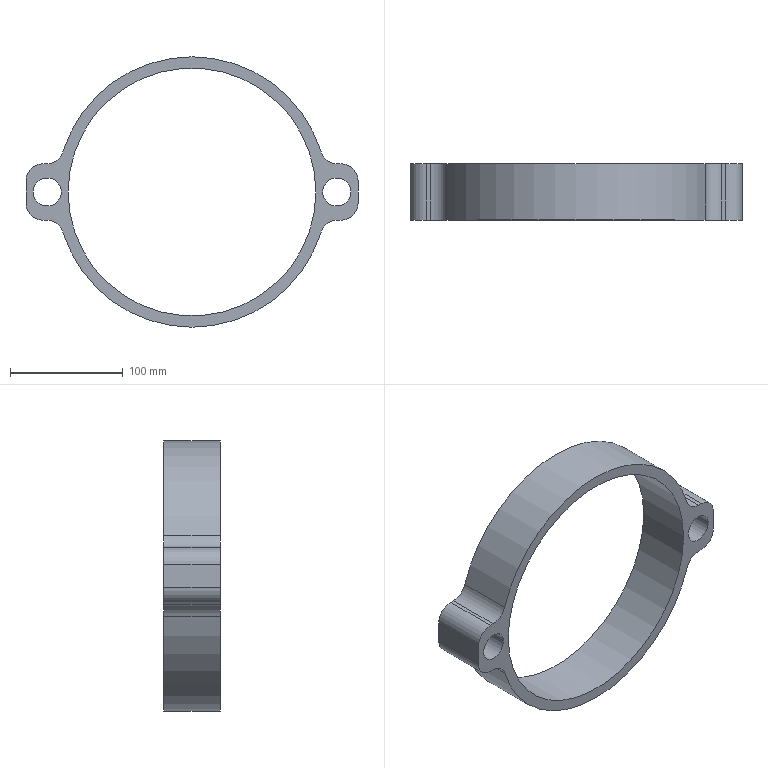Part | NX | features BREP 1 | 1 solid | 24 faces | box 294.734 x 50 x 240 mm | volume 448691 mm3 | cylinder 16 | plane 8 | commonest cylinder face diameters 30 x8 25 x4 220 x2 240 x2
STEP:
#1=CARTESIAN_POINT('',(-128.938,0.,-25.));
#2=VERTEX_POINT('',#1);
#3=CARTESIAN_POINT('',(-132.367,0.,-25.));
#4=VERTEX_POINT('',#3);
#5=CARTESIAN_POINT('',(-128.938,0.,-25.));
#6=DIRECTION('',(-1.,0.,0.));
#7=VECTOR('',#6,1000.);
#8=LINE('',#5,#7);
#9=EDGE_CURVE('',#2,#4,#8,.T.);
#10=ORIENTED_EDGE('',*,*,#9,.F.);
#11=CARTESIAN_POINT('',(-114.612,0.,-35.556));
#12=VERTEX_POINT('',#11);
#13=CARTESIAN_POINT('',(-128.938,0.,-40.));
#14=DIRECTION('',(0.,1.,0.));
#15=DIRECTION('',(0.,0.,1.));
#16=AXIS2_PLACEMENT_3D('',#13,#14,#15);
#17=CIRCLE('',#16,15.);
#18=EDGE_CURVE('',#2,#12,#17,.T.);
#19=ORIENTED_EDGE('',*,*,#18,.T.);
#20=CARTESIAN_POINT('',(114.612,0.,-35.556));
#21=VERTEX_POINT('',#20);
#22=CARTESIAN_POINT('',(0.,0.,0.));
#23=DIRECTION('',(0.,1.,0.));
#24=DIRECTION('',(0.9551,0.,-0.2963));
#25=AXIS2_PLACEMENT_3D('',#22,#23,#24);
#26=CIRCLE('',#25,120.);
#27=EDGE_CURVE('',#21,#12,#26,.T.);
#28=ORIENTED_EDGE('',*,*,#27,.F.);
#29=CARTESIAN_POINT('',(128.938,0.,-25.));
#30=VERTEX_POINT('',#29);
#31=CARTESIAN_POINT('',(128.938,0.,-40.));
#32=DIRECTION('',(0.,1.,0.));
#33=DIRECTION('',(-0.9551,0.,0.2963));
#34=AXIS2_PLACEMENT_3D('',#31,#32,#33);
#35=CIRCLE('',#34,15.);
#36=EDGE_CURVE('',#21,#30,#35,.T.);
#37=ORIENTED_EDGE('',*,*,#36,.T.);
#38=CARTESIAN_POINT('',(132.367,0.,-25.));
#39=VERTEX_POINT('',#38);
#40=CARTESIAN_POINT('',(132.367,0.,-25.));
#41=DIRECTION('',(-1.,0.,0.));
#42=VECTOR('',#41,1000.);
#43=LINE('',#40,#42);
#44=EDGE_CURVE('',#39,#30,#43,.T.);
#45=ORIENTED_EDGE('',*,*,#44,.F.);
#46=CARTESIAN_POINT('',(147.367,0.,-10.));
#47=VERTEX_POINT('',#46);
#48=CARTESIAN_POINT('',(132.367,0.,-10.));
#49=DIRECTION('',(0.,-1.,0.));
#50=DIRECTION('',(0.,0.,-1.));
#51=AXIS2_PLACEMENT_3D('',#48,#49,#50);
#52=CIRCLE('',#51,15.);
#53=EDGE_CURVE('',#39,#47,#52,.T.);
#54=ORIENTED_EDGE('',*,*,#53,.T.);
#55=CARTESIAN_POINT('',(147.367,0.,10.));
#56=VERTEX_POINT('',#55);
#57=CARTESIAN_POINT('',(147.367,0.,10.));
#58=DIRECTION('',(0.,0.,-1.));
#59=VECTOR('',#58,1000.);
#60=LINE('',#57,#59);
#61=EDGE_CURVE('',#56,#47,#60,.T.);
#62=ORIENTED_EDGE('',*,*,#61,.F.);
#63=CARTESIAN_POINT('',(132.367,0.,25.));
#64=VERTEX_POINT('',#63);
#65=CARTESIAN_POINT('',(132.367,0.,10.));
#66=DIRECTION('',(0.,-1.,0.));
#67=DIRECTION('',(1.,0.,0.));
#68=AXIS2_PLACEMENT_3D('',#65,#66,#67);
#69=CIRCLE('',#68,15.);
#70=EDGE_CURVE('',#56,#64,#69,.T.);
#71=ORIENTED_EDGE('',*,*,#70,.T.);
#72=CARTESIAN_POINT('',(128.938,0.,25.));
#73=VERTEX_POINT('',#72);
#74=CARTESIAN_POINT('',(128.938,0.,25.));
#75=DIRECTION('',(1.,0.,0.));
#76=VECTOR('',#75,1000.);
#77=LINE('',#74,#76);
#78=EDGE_CURVE('',#73,#64,#77,.T.);
#79=ORIENTED_EDGE('',*,*,#78,.F.);
#80=CARTESIAN_POINT('',(114.612,0.,35.556));
#81=VERTEX_POINT('',#80);
#82=CARTESIAN_POINT('',(128.938,0.,40.));
#83=DIRECTION('',(0.,1.,0.));
#84=DIRECTION('',(0.,0.,-1.));
#85=AXIS2_PLACEMENT_3D('',#82,#83,#84);
#86=CIRCLE('',#85,15.);
#87=EDGE_CURVE('',#73,#81,#86,.T.);
#88=ORIENTED_EDGE('',*,*,#87,.T.);
#89=CARTESIAN_POINT('',(-114.612,0.,35.556));
#90=VERTEX_POINT('',#89);
#91=CARTESIAN_POINT('',(0.,0.,0.));
#92=DIRECTION('',(0.,1.,0.));
#93=DIRECTION('',(-0.9551,0.,0.2963));
#94=AXIS2_PLACEMENT_3D('',#91,#92,#93);
#95=CIRCLE('',#94,120.);
#96=EDGE_CURVE('',#90,#81,#95,.T.);
#97=ORIENTED_EDGE('',*,*,#96,.F.);
#98=CARTESIAN_POINT('',(-128.938,0.,25.));
#99=VERTEX_POINT('',#98);
#100=CARTESIAN_POINT('',(-128.938,0.,40.));
#101=DIRECTION('',(0.,1.,0.));
#102=DIRECTION('',(0.9551,0.,-0.2963));
#103=AXIS2_PLACEMENT_3D('',#100,#101,#102);
#104=CIRCLE('',#103,15.);
#105=EDGE_CURVE('',#90,#99,#104,.T.);
#106=ORIENTED_EDGE('',*,*,#105,.T.);
#107=CARTESIAN_POINT('',(-132.367,0.,25.));
#108=VERTEX_POINT('',#107);
#109=CARTESIAN_POINT('',(-132.367,0.,25.));
#110=DIRECTION('',(1.,0.,0.));
#111=VECTOR('',#110,1000.);
#112=LINE('',#109,#111);
#113=EDGE_CURVE('',#108,#99,#112,.T.);
#114=ORIENTED_EDGE('',*,*,#113,.F.);
#115=CARTESIAN_POINT('',(-147.367,0.,10.));
#116=VERTEX_POINT('',#115);
#117=CARTESIAN_POINT('',(-132.367,0.,10.));
#118=DIRECTION('',(0.,-1.,0.));
#119=DIRECTION('',(0.,0.,1.));
#120=AXIS2_PLACEMENT_3D('',#117,#118,#119);
#121=CIRCLE('',#120,15.);
#122=EDGE_CURVE('',#108,#116,#121,.T.);
#123=ORIENTED_EDGE('',*,*,#122,.T.);
#124=CARTESIAN_POINT('',(-147.367,0.,-10.));
#125=VERTEX_POINT('',#124);
#126=CARTESIAN_POINT('',(-147.367,0.,-10.));
#127=DIRECTION('',(0.,0.,1.));
#128=VECTOR('',#127,1000.);
#129=LINE('',#126,#128);
#130=EDGE_CURVE('',#125,#116,#129,.T.);
#131=ORIENTED_EDGE('',*,*,#130,.F.);
#132=CARTESIAN_POINT('',(-132.367,0.,-10.));
#133=DIRECTION('',(0.,-1.,0.));
#134=DIRECTION('',(-1.,0.,0.));
#135=AXIS2_PLACEMENT_3D('',#132,#133,#134);
#136=CIRCLE('',#135,15.);
#137=EDGE_CURVE('',#125,#4,#136,.T.);
#138=ORIENTED_EDGE('',*,*,#137,.T.);
#139=EDGE_LOOP('',(#10,#19,#28,#37,#45,#54,#62,#71,#79,#88,#97,#106,#114,#123,#131,#138));
#140=FACE_BOUND('',#139,.T.);
#141=CARTESIAN_POINT('',(-110.,0.,0.));
#142=VERTEX_POINT('',#141);
#143=CARTESIAN_POINT('',(110.,0.,0.));
#144=VERTEX_POINT('',#143);
#145=CARTESIAN_POINT('',(0.,0.,0.));
#146=DIRECTION('',(0.,-1.,0.));
#147=DIRECTION('',(-1.,0.,0.));
#148=AXIS2_PLACEMENT_3D('',#145,#146,#147);
#149=CIRCLE('',#148,110.);
#150=EDGE_CURVE('',#142,#144,#149,.T.);
#151=ORIENTED_EDGE('',*,*,#150,.F.);
#152=CARTESIAN_POINT('',(0.,0.,0.));
#153=DIRECTION('',(0.,-1.,0.));
#154=DIRECTION('',(1.,0.,0.));
#155=AXIS2_PLACEMENT_3D('',#152,#153,#154);
#156=CIRCLE('',#155,110.);
#157=EDGE_CURVE('',#144,#142,#156,.T.);
#158=ORIENTED_EDGE('',*,*,#157,.F.);
#159=EDGE_LOOP('',(#151,#158));
#160=FACE_BOUND('',#159,.T.);
#161=CARTESIAN_POINT('',(-141.,0.,0.));
#162=VERTEX_POINT('',#161);
#163=CARTESIAN_POINT('',(-116.,0.,0.));
#164=VERTEX_POINT('',#163);
#165=CARTESIAN_POINT('',(-128.5,0.,0.));
#166=DIRECTION('',(0.,1.,0.));
#167=DIRECTION('',(-1.,0.,0.));
#168=AXIS2_PLACEMENT_3D('',#165,#166,#167);
#169=CIRCLE('',#168,12.5);
#170=EDGE_CURVE('',#162,#164,#169,.T.);
#171=ORIENTED_EDGE('',*,*,#170,.T.);
#172=CARTESIAN_POINT('',(-128.5,0.,0.));
#173=DIRECTION('',(0.,1.,0.));
#174=DIRECTION('',(1.,0.,0.));
#175=AXIS2_PLACEMENT_3D('',#172,#173,#174);
#176=CIRCLE('',#175,12.5);
#177=EDGE_CURVE('',#164,#162,#176,.T.);
#178=ORIENTED_EDGE('',*,*,#177,.T.);
#179=EDGE_LOOP('',(#171,#178));
#180=FACE_BOUND('',#179,.T.);
#181=CARTESIAN_POINT('',(116.,0.,0.));
#182=VERTEX_POINT('',#181);
#183=CARTESIAN_POINT('',(141.,0.,0.));
#184=VERTEX_POINT('',#183);
#185=CARTESIAN_POINT('',(128.5,0.,0.));
#186=DIRECTION('',(0.,1.,0.));
#187=DIRECTION('',(-1.,0.,0.));
#188=AXIS2_PLACEMENT_3D('',#185,#186,#187);
#189=CIRCLE('',#188,12.5);
#190=EDGE_CURVE('',#182,#184,#189,.T.);
#191=ORIENTED_EDGE('',*,*,#190,.T.);
#192=CARTESIAN_POINT('',(128.5,0.,0.));
#193=DIRECTION('',(0.,1.,0.));
#194=DIRECTION('',(1.,0.,0.));
#195=AXIS2_PLACEMENT_3D('',#192,#193,#194);
#196=CIRCLE('',#195,12.5);
#197=EDGE_CURVE('',#184,#182,#196,.T.);
#198=ORIENTED_EDGE('',*,*,#197,.T.);
#199=EDGE_LOOP('',(#191,#198));
#200=FACE_BOUND('',#199,.T.);
#201=CARTESIAN_POINT('',(0.,0.,0.));
#202=DIRECTION('',(0.,1.,0.));
#203=DIRECTION('',(1.,0.,0.));
#204=AXIS2_PLACEMENT_3D('',#201,#202,#203);
#205=PLANE('',#204);
#206=ADVANCED_FACE('',(#140,#160,#180,#200),#205,.F.);
#207=CARTESIAN_POINT('',(-110.,50.,0.));
#208=VERTEX_POINT('',#207);
#209=CARTESIAN_POINT('',(-110.,0.,0.));
#210=DIRECTION('',(0.,1.,0.));
#211=VECTOR('',#210,1000.);
#212=LINE('',#209,#211);
#213=EDGE_CURVE('',#142,#208,#212,.T.);
#214=ORIENTED_EDGE('',*,*,#213,.T.);
#215=CARTESIAN_POINT('',(110.,50.,0.));
#216=VERTEX_POINT('',#215);
#217=CARTESIAN_POINT('',(0.,50.,0.));
#218=DIRECTION('',(0.,-1.,0.));
#219=DIRECTION('',(1.,0.,0.));
#220=AXIS2_PLACEMENT_3D('',#217,#218,#219);
#221=CIRCLE('',#220,110.);
#222=EDGE_CURVE('',#216,#208,#221,.T.);
#223=ORIENTED_EDGE('',*,*,#222,.F.);
#224=CARTESIAN_POINT('',(110.,0.,0.));
#225=DIRECTION('',(0.,1.,0.));
#226=VECTOR('',#225,1000.);
#227=LINE('',#224,#226);
#228=EDGE_CURVE('',#144,#216,#227,.T.);
#229=ORIENTED_EDGE('',*,*,#228,.F.);
#230=ORIENTED_EDGE('',*,*,#157,.T.);
#231=EDGE_LOOP('',(#214,#223,#229,#230));
#232=FACE_BOUND('',#231,.T.);
#233=CARTESIAN_POINT('',(0.,0.,0.));
#234=DIRECTION('',(0.,1.,0.));
#235=DIRECTION('',(1.,0.,0.));
#236=AXIS2_PLACEMENT_3D('',#233,#234,#235);
#237=CYLINDRICAL_SURFACE('',#236,110.);
#238=ADVANCED_FACE('',(#232),#237,.F.);
#239=ORIENTED_EDGE('',*,*,#228,.T.);
#240=CARTESIAN_POINT('',(0.,50.,0.));
#241=DIRECTION('',(0.,-1.,0.));
#242=DIRECTION('',(-1.,0.,0.));
#243=AXIS2_PLACEMENT_3D('',#240,#241,#242);
#244=CIRCLE('',#243,110.);
#245=EDGE_CURVE('',#208,#216,#244,.T.);
#246=ORIENTED_EDGE('',*,*,#245,.F.);
#247=ORIENTED_EDGE('',*,*,#213,.F.);
#248=ORIENTED_EDGE('',*,*,#150,.T.);
#249=EDGE_LOOP('',(#239,#246,#247,#248));
#250=FACE_BOUND('',#249,.T.);
#251=CARTESIAN_POINT('',(0.,0.,0.));
#252=DIRECTION('',(0.,1.,0.));
#253=DIRECTION('',(1.,0.,0.));
#254=AXIS2_PLACEMENT_3D('',#251,#252,#253);
#255=CYLINDRICAL_SURFACE('',#254,110.);
#256=ADVANCED_FACE('',(#250),#255,.F.);
#257=CARTESIAN_POINT('',(-147.367,50.,-10.));
#258=VERTEX_POINT('',#257);
#259=CARTESIAN_POINT('',(-147.367,50.,10.));
#260=VERTEX_POINT('',#259);
#261=CARTESIAN_POINT('',(-147.367,50.,-10.));
#262=DIRECTION('',(0.,0.,1.));
#263=VECTOR('',#262,1000.);
#264=LINE('',#261,#263);
#265=EDGE_CURVE('',#258,#260,#264,.T.);
#266=ORIENTED_EDGE('',*,*,#265,.T.);
#267=CARTESIAN_POINT('',(-132.367,50.,25.));
#268=VERTEX_POINT('',#267);
#269=CARTESIAN_POINT('',(-132.367,50.,10.));
#270=DIRECTION('',(0.,1.,0.));
#271=DIRECTION('',(-1.,0.,0.));
#272=AXIS2_PLACEMENT_3D('',#269,#270,#271);
#273=CIRCLE('',#272,15.);
#274=EDGE_CURVE('',#260,#268,#273,.T.);
#275=ORIENTED_EDGE('',*,*,#274,.T.);
#276=CARTESIAN_POINT('',(-128.938,50.,25.));
#277=VERTEX_POINT('',#276);
#278=CARTESIAN_POINT('',(-132.367,50.,25.));
#279=DIRECTION('',(1.,0.,0.));
#280=VECTOR('',#279,1000.);
#281=LINE('',#278,#280);
#282=EDGE_CURVE('',#268,#277,#281,.T.);
#283=ORIENTED_EDGE('',*,*,#282,.T.);
#284=CARTESIAN_POINT('',(-114.612,50.,35.556));
#285=VERTEX_POINT('',#284);
#286=CARTESIAN_POINT('',(-128.938,50.,40.));
#287=DIRECTION('',(0.,-1.,0.));
#288=DIRECTION('',(0.,0.,-1.));
#289=AXIS2_PLACEMENT_3D('',#286,#287,#288);
#290=CIRCLE('',#289,15.);
#291=EDGE_CURVE('',#277,#285,#290,.T.);
#292=ORIENTED_EDGE('',*,*,#291,.T.);
#293=CARTESIAN_POINT('',(114.612,50.,35.556));
#294=VERTEX_POINT('',#293);
#295=CARTESIAN_POINT('',(0.,50.,0.));
#296=DIRECTION('',(0.,1.,0.));
#297=DIRECTION('',(-0.9551,0.,0.2963));
#298=AXIS2_PLACEMENT_3D('',#295,#296,#297);
#299=CIRCLE('',#298,120.);
#300=EDGE_CURVE('',#285,#294,#299,.T.);
#301=ORIENTED_EDGE('',*,*,#300,.T.);
#302=CARTESIAN_POINT('',(128.938,50.,25.));
#303=VERTEX_POINT('',#302);
#304=CARTESIAN_POINT('',(128.938,50.,40.));
#305=DIRECTION('',(0.,-1.,0.));
#306=DIRECTION('',(-0.9551,0.,-0.2963));
#307=AXIS2_PLACEMENT_3D('',#304,#305,#306);
#308=CIRCLE('',#307,15.);
#309=EDGE_CURVE('',#294,#303,#308,.T.);
#310=ORIENTED_EDGE('',*,*,#309,.T.);
#311=CARTESIAN_POINT('',(132.367,50.,25.));
#312=VERTEX_POINT('',#311);
#313=CARTESIAN_POINT('',(128.938,50.,25.));
#314=DIRECTION('',(1.,0.,0.));
#315=VECTOR('',#314,1000.);
#316=LINE('',#313,#315);
#317=EDGE_CURVE('',#303,#312,#316,.T.);
#318=ORIENTED_EDGE('',*,*,#317,.T.);
#319=CARTESIAN_POINT('',(147.367,50.,10.));
#320=VERTEX_POINT('',#319);
#321=CARTESIAN_POINT('',(132.367,50.,10.));
#322=DIRECTION('',(0.,1.,0.));
#323=DIRECTION('',(0.,0.,1.));
#324=AXIS2_PLACEMENT_3D('',#321,#322,#323);
#325=CIRCLE('',#324,15.);
#326=EDGE_CURVE('',#312,#320,#325,.T.);
#327=ORIENTED_EDGE('',*,*,#326,.T.);
#328=CARTESIAN_POINT('',(147.367,50.,-10.));
#329=VERTEX_POINT('',#328);
#330=CARTESIAN_POINT('',(147.367,50.,10.));
#331=DIRECTION('',(0.,0.,-1.));
#332=VECTOR('',#331,1000.);
#333=LINE('',#330,#332);
#334=EDGE_CURVE('',#320,#329,#333,.T.);
#335=ORIENTED_EDGE('',*,*,#334,.T.);
#336=CARTESIAN_POINT('',(132.367,50.,-25.));
#337=VERTEX_POINT('',#336);
#338=CARTESIAN_POINT('',(132.367,50.,-10.));
#339=DIRECTION('',(0.,1.,0.));
#340=DIRECTION('',(1.,0.,0.));
#341=AXIS2_PLACEMENT_3D('',#338,#339,#340);
#342=CIRCLE('',#341,15.);
#343=EDGE_CURVE('',#329,#337,#342,.T.);
#344=ORIENTED_EDGE('',*,*,#343,.T.);
#345=CARTESIAN_POINT('',(128.938,50.,-25.));
#346=VERTEX_POINT('',#345);
#347=CARTESIAN_POINT('',(132.367,50.,-25.));
#348=DIRECTION('',(-1.,0.,0.));
#349=VECTOR('',#348,1000.);
#350=LINE('',#347,#349);
#351=EDGE_CURVE('',#337,#346,#350,.T.);
#352=ORIENTED_EDGE('',*,*,#351,.T.);
#353=CARTESIAN_POINT('',(114.612,50.,-35.556));
#354=VERTEX_POINT('',#353);
#355=CARTESIAN_POINT('',(128.938,50.,-40.));
#356=DIRECTION('',(0.,-1.,0.));
#357=DIRECTION('',(0.,0.,1.));
#358=AXIS2_PLACEMENT_3D('',#355,#356,#357);
#359=CIRCLE('',#358,15.);
#360=EDGE_CURVE('',#346,#354,#359,.T.);
#361=ORIENTED_EDGE('',*,*,#360,.T.);
#362=CARTESIAN_POINT('',(-114.612,50.,-35.556));
#363=VERTEX_POINT('',#362);
#364=CARTESIAN_POINT('',(0.,50.,0.));
#365=DIRECTION('',(0.,1.,0.));
#366=DIRECTION('',(0.9551,0.,-0.2963));
#367=AXIS2_PLACEMENT_3D('',#364,#365,#366);
#368=CIRCLE('',#367,120.);
#369=EDGE_CURVE('',#354,#363,#368,.T.);
#370=ORIENTED_EDGE('',*,*,#369,.T.);
#371=CARTESIAN_POINT('',(-128.938,50.,-25.));
#372=VERTEX_POINT('',#371);
#373=CARTESIAN_POINT('',(-128.938,50.,-40.));
#374=DIRECTION('',(0.,-1.,0.));
#375=DIRECTION('',(0.9551,0.,0.2963));
#376=AXIS2_PLACEMENT_3D('',#373,#374,#375);
#377=CIRCLE('',#376,15.);
#378=EDGE_CURVE('',#363,#372,#377,.T.);
#379=ORIENTED_EDGE('',*,*,#378,.T.);
#380=CARTESIAN_POINT('',(-132.367,50.,-25.));
#381=VERTEX_POINT('',#380);
#382=CARTESIAN_POINT('',(-128.938,50.,-25.));
#383=DIRECTION('',(-1.,0.,0.));
#384=VECTOR('',#383,1000.);
#385=LINE('',#382,#384);
#386=EDGE_CURVE('',#372,#381,#385,.T.);
#387=ORIENTED_EDGE('',*,*,#386,.T.);
#388=CARTESIAN_POINT('',(-132.367,50.,-10.));
#389=DIRECTION('',(0.,1.,0.));
#390=DIRECTION('',(0.,0.,-1.));
#391=AXIS2_PLACEMENT_3D('',#388,#389,#390);
#392=CIRCLE('',#391,15.);
#393=EDGE_CURVE('',#381,#258,#392,.T.);
#394=ORIENTED_EDGE('',*,*,#393,.T.);
#395=EDGE_LOOP('',(#266,#275,#283,#292,#301,#310,#318,#327,#335,#344,#352,#361,#370,#379,#387,#394));
#396=FACE_BOUND('',#395,.T.);
#397=ORIENTED_EDGE('',*,*,#245,.T.);
#398=ORIENTED_EDGE('',*,*,#222,.T.);
#399=EDGE_LOOP('',(#397,#398));
#400=FACE_BOUND('',#399,.T.);
#401=CARTESIAN_POINT('',(-141.,50.,0.));
#402=VERTEX_POINT('',#401);
#403=CARTESIAN_POINT('',(-116.,50.,0.));
#404=VERTEX_POINT('',#403);
#405=CARTESIAN_POINT('',(-128.5,50.,0.));
#406=DIRECTION('',(0.,1.,0.));
#407=DIRECTION('',(-1.,0.,0.));
#408=AXIS2_PLACEMENT_3D('',#405,#406,#407);
#409=CIRCLE('',#408,12.5);
#410=EDGE_CURVE('',#402,#404,#409,.T.);
#411=ORIENTED_EDGE('',*,*,#410,.F.);
#412=CARTESIAN_POINT('',(-128.5,50.,0.));
#413=DIRECTION('',(0.,1.,0.));
#414=DIRECTION('',(1.,0.,0.));
#415=AXIS2_PLACEMENT_3D('',#412,#413,#414);
#416=CIRCLE('',#415,12.5);
#417=EDGE_CURVE('',#404,#402,#416,.T.);
#418=ORIENTED_EDGE('',*,*,#417,.F.);
#419=EDGE_LOOP('',(#411,#418));
#420=FACE_BOUND('',#419,.T.);
#421=CARTESIAN_POINT('',(116.,50.,0.));
#422=VERTEX_POINT('',#421);
#423=CARTESIAN_POINT('',(141.,50.,0.));
#424=VERTEX_POINT('',#423);
#425=CARTESIAN_POINT('',(128.5,50.,0.));
#426=DIRECTION('',(0.,1.,0.));
#427=DIRECTION('',(-1.,0.,0.));
#428=AXIS2_PLACEMENT_3D('',#425,#426,#427);
#429=CIRCLE('',#428,12.5);
#430=EDGE_CURVE('',#422,#424,#429,.T.);
#431=ORIENTED_EDGE('',*,*,#430,.F.);
#432=CARTESIAN_POINT('',(128.5,50.,0.));
#433=DIRECTION('',(0.,1.,0.));
#434=DIRECTION('',(1.,0.,0.));
#435=AXIS2_PLACEMENT_3D('',#432,#433,#434);
#436=CIRCLE('',#435,12.5);
#437=EDGE_CURVE('',#424,#422,#436,.T.);
#438=ORIENTED_EDGE('',*,*,#437,.F.);
#439=EDGE_LOOP('',(#431,#438));
#440=FACE_BOUND('',#439,.T.);
#441=CARTESIAN_POINT('',(0.,50.,0.));
#442=DIRECTION('',(0.,1.,0.));
#443=DIRECTION('',(1.,0.,0.));
#444=AXIS2_PLACEMENT_3D('',#441,#442,#443);
#445=PLANE('',#444);
#446=ADVANCED_FACE('',(#396,#400,#420,#440),#445,.T.);
#447=CARTESIAN_POINT('',(-147.367,50.,-10.));
#448=DIRECTION('',(0.,-1.,0.));
#449=VECTOR('',#448,1000.);
#450=LINE('',#447,#449);
#451=EDGE_CURVE('',#258,#125,#450,.T.);
#452=ORIENTED_EDGE('',*,*,#451,.F.);
#453=ORIENTED_EDGE('',*,*,#393,.F.);
#454=CARTESIAN_POINT('',(-132.367,50.,-25.));
#455=DIRECTION('',(0.,-1.,0.));
#456=VECTOR('',#455,1000.);
#457=LINE('',#454,#456);
#458=EDGE_CURVE('',#381,#4,#457,.T.);
#459=ORIENTED_EDGE('',*,*,#458,.T.);
#460=ORIENTED_EDGE('',*,*,#137,.F.);
#461=EDGE_LOOP('',(#452,#453,#459,#460));
#462=FACE_BOUND('',#461,.T.);
#463=CARTESIAN_POINT('',(-132.367,115.18,-10.));
#464=DIRECTION('',(0.,-1.,0.));
#465=DIRECTION('',(-1.,0.,0.));
#466=AXIS2_PLACEMENT_3D('',#463,#464,#465);
#467=CYLINDRICAL_SURFACE('',#466,15.);
#468=ADVANCED_FACE('',(#462),#467,.T.);
#469=ORIENTED_EDGE('',*,*,#386,.F.);
#470=CARTESIAN_POINT('',(-128.938,0.,-25.));
#471=DIRECTION('',(0.,1.,0.));
#472=VECTOR('',#471,1000.);
#473=LINE('',#470,#472);
#474=EDGE_CURVE('',#2,#372,#473,.T.);
#475=ORIENTED_EDGE('',*,*,#474,.F.);
#476=ORIENTED_EDGE('',*,*,#9,.T.);
#477=ORIENTED_EDGE('',*,*,#458,.F.);
#478=EDGE_LOOP('',(#469,#475,#476,#477));
#479=FACE_BOUND('',#478,.T.);
#480=CARTESIAN_POINT('',(-117.367,0.,-25.));
#481=DIRECTION('',(0.,0.,-1.));
#482=DIRECTION('',(0.,-1.,0.));
#483=AXIS2_PLACEMENT_3D('',#480,#481,#482);
#484=PLANE('',#483);
#485=ADVANCED_FACE('',(#479),#484,.T.);
#486=ORIENTED_EDGE('',*,*,#378,.F.);
#487=CARTESIAN_POINT('',(-114.612,0.,-35.556));
#488=DIRECTION('',(0.,1.,0.));
#489=VECTOR('',#488,1000.);
#490=LINE('',#487,#489);
#491=EDGE_CURVE('',#12,#363,#490,.T.);
#492=ORIENTED_EDGE('',*,*,#491,.F.);
#493=ORIENTED_EDGE('',*,*,#18,.F.);
#494=ORIENTED_EDGE('',*,*,#474,.T.);
#495=EDGE_LOOP('',(#486,#492,#493,#494));
#496=FACE_BOUND('',#495,.T.);
#497=CARTESIAN_POINT('',(-128.938,-65.18,-40.));
#498=DIRECTION('',(0.,1.,0.));
#499=DIRECTION('',(0.,0.,1.));
#500=AXIS2_PLACEMENT_3D('',#497,#498,#499);
#501=CYLINDRICAL_SURFACE('',#500,15.);
#502=ADVANCED_FACE('',(#496),#501,.F.);
#503=ORIENTED_EDGE('',*,*,#369,.F.);
#504=CARTESIAN_POINT('',(114.612,0.,-35.556));
#505=DIRECTION('',(0.,1.,0.));
#506=VECTOR('',#505,1000.);
#507=LINE('',#504,#506);
#508=EDGE_CURVE('',#21,#354,#507,.T.);
#509=ORIENTED_EDGE('',*,*,#508,.F.);
#510=ORIENTED_EDGE('',*,*,#27,.T.);
#511=ORIENTED_EDGE('',*,*,#491,.T.);
#512=EDGE_LOOP('',(#503,#509,#510,#511));
#513=FACE_BOUND('',#512,.T.);
#514=CARTESIAN_POINT('',(0.,0.,0.));
#515=DIRECTION('',(0.,1.,0.));
#516=DIRECTION('',(1.,0.,0.));
#517=AXIS2_PLACEMENT_3D('',#514,#515,#516);
#518=CYLINDRICAL_SURFACE('',#517,120.);
#519=ADVANCED_FACE('',(#513),#518,.T.);
#520=ORIENTED_EDGE('',*,*,#360,.F.);
#521=CARTESIAN_POINT('',(128.938,0.,-25.));
#522=DIRECTION('',(0.,1.,0.));
#523=VECTOR('',#522,1000.);
#524=LINE('',#521,#523);
#525=EDGE_CURVE('',#30,#346,#524,.T.);
#526=ORIENTED_EDGE('',*,*,#525,.F.);
#527=ORIENTED_EDGE('',*,*,#36,.F.);
#528=ORIENTED_EDGE('',*,*,#508,.T.);
#529=EDGE_LOOP('',(#520,#526,#527,#528));
#530=FACE_BOUND('',#529,.T.);
#531=CARTESIAN_POINT('',(128.938,-65.18,-40.));
#532=DIRECTION('',(0.,1.,0.));
#533=DIRECTION('',(-0.9551,0.,0.2963));
#534=AXIS2_PLACEMENT_3D('',#531,#532,#533);
#535=CYLINDRICAL_SURFACE('',#534,15.);
#536=ADVANCED_FACE('',(#530),#535,.F.);
#537=ORIENTED_EDGE('',*,*,#44,.T.);
#538=ORIENTED_EDGE('',*,*,#525,.T.);
#539=ORIENTED_EDGE('',*,*,#351,.F.);
#540=CARTESIAN_POINT('',(132.367,50.,-25.));
#541=DIRECTION('',(0.,-1.,0.));
#542=VECTOR('',#541,1000.);
#543=LINE('',#540,#542);
#544=EDGE_CURVE('',#337,#39,#543,.T.);
#545=ORIENTED_EDGE('',*,*,#544,.T.);
#546=EDGE_LOOP('',(#537,#538,#539,#545));
#547=FACE_BOUND('',#546,.T.);
#548=CARTESIAN_POINT('',(147.367,0.,-25.));
#549=DIRECTION('',(0.,0.,-1.));
#550=DIRECTION('',(0.,-1.,0.));
#551=AXIS2_PLACEMENT_3D('',#548,#549,#550);
#552=PLANE('',#551);
#553=ADVANCED_FACE('',(#547),#552,.T.);
#554=ORIENTED_EDGE('',*,*,#544,.F.);
#555=ORIENTED_EDGE('',*,*,#343,.F.);
#556=CARTESIAN_POINT('',(147.367,50.,-10.));
#557=DIRECTION('',(0.,-1.,0.));
#558=VECTOR('',#557,1000.);
#559=LINE('',#556,#558);
#560=EDGE_CURVE('',#329,#47,#559,.T.);
#561=ORIENTED_EDGE('',*,*,#560,.T.);
#562=ORIENTED_EDGE('',*,*,#53,.F.);
#563=EDGE_LOOP('',(#554,#555,#561,#562));
#564=FACE_BOUND('',#563,.T.);
#565=CARTESIAN_POINT('',(132.367,115.18,-10.));
#566=DIRECTION('',(0.,-1.,0.));
#567=DIRECTION('',(0.,0.,-1.));
#568=AXIS2_PLACEMENT_3D('',#565,#566,#567);
#569=CYLINDRICAL_SURFACE('',#568,15.);
#570=ADVANCED_FACE('',(#564),#569,.T.);
#571=ORIENTED_EDGE('',*,*,#61,.T.);
#572=ORIENTED_EDGE('',*,*,#560,.F.);
#573=ORIENTED_EDGE('',*,*,#334,.F.);
#574=CARTESIAN_POINT('',(147.367,50.,10.));
#575=DIRECTION('',(0.,-1.,0.));
#576=VECTOR('',#575,1000.);
#577=LINE('',#574,#576);
#578=EDGE_CURVE('',#320,#56,#577,.T.);
#579=ORIENTED_EDGE('',*,*,#578,.T.);
#580=EDGE_LOOP('',(#571,#572,#573,#579));
#581=FACE_BOUND('',#580,.T.);
#582=CARTESIAN_POINT('',(147.367,0.,25.));
#583=DIRECTION('',(1.,0.,0.));
#584=DIRECTION('',(0.,1.,0.));
#585=AXIS2_PLACEMENT_3D('',#582,#583,#584);
#586=PLANE('',#585);
#587=ADVANCED_FACE('',(#581),#586,.T.);
#588=ORIENTED_EDGE('',*,*,#578,.F.);
#589=ORIENTED_EDGE('',*,*,#326,.F.);
#590=CARTESIAN_POINT('',(132.367,50.,25.));
#591=DIRECTION('',(0.,-1.,0.));
#592=VECTOR('',#591,1000.);
#593=LINE('',#590,#592);
#594=EDGE_CURVE('',#312,#64,#593,.T.);
#595=ORIENTED_EDGE('',*,*,#594,.T.);
#596=ORIENTED_EDGE('',*,*,#70,.F.);
#597=EDGE_LOOP('',(#588,#589,#595,#596));
#598=FACE_BOUND('',#597,.T.);
#599=CARTESIAN_POINT('',(132.367,115.18,10.));
#600=DIRECTION('',(0.,-1.,0.));
#601=DIRECTION('',(1.,0.,0.));
#602=AXIS2_PLACEMENT_3D('',#599,#600,#601);
#603=CYLINDRICAL_SURFACE('',#602,15.);
#604=ADVANCED_FACE('',(#598),#603,.T.);
#605=ORIENTED_EDGE('',*,*,#317,.F.);
#606=CARTESIAN_POINT('',(128.938,0.,25.));
#607=DIRECTION('',(0.,1.,0.));
#608=VECTOR('',#607,1000.);
#609=LINE('',#606,#608);
#610=EDGE_CURVE('',#73,#303,#609,.T.);
#611=ORIENTED_EDGE('',*,*,#610,.F.);
#612=ORIENTED_EDGE('',*,*,#78,.T.);
#613=ORIENTED_EDGE('',*,*,#594,.F.);
#614=EDGE_LOOP('',(#605,#611,#612,#613));
#615=FACE_BOUND('',#614,.T.);
#616=CARTESIAN_POINT('',(117.367,0.,25.));
#617=DIRECTION('',(0.,0.,1.));
#618=DIRECTION('',(1.,0.,0.));
#619=AXIS2_PLACEMENT_3D('',#616,#617,#618);
#620=PLANE('',#619);
#621=ADVANCED_FACE('',(#615),#620,.T.);
#622=ORIENTED_EDGE('',*,*,#309,.F.);
#623=CARTESIAN_POINT('',(114.612,0.,35.556));
#624=DIRECTION('',(0.,1.,0.));
#625=VECTOR('',#624,1000.);
#626=LINE('',#623,#625);
#627=EDGE_CURVE('',#81,#294,#626,.T.);
#628=ORIENTED_EDGE('',*,*,#627,.F.);
#629=ORIENTED_EDGE('',*,*,#87,.F.);
#630=ORIENTED_EDGE('',*,*,#610,.T.);
#631=EDGE_LOOP('',(#622,#628,#629,#630));
#632=FACE_BOUND('',#631,.T.);
#633=CARTESIAN_POINT('',(128.938,-65.18,40.));
#634=DIRECTION('',(0.,1.,0.));
#635=DIRECTION('',(0.,0.,-1.));
#636=AXIS2_PLACEMENT_3D('',#633,#634,#635);
#637=CYLINDRICAL_SURFACE('',#636,15.);
#638=ADVANCED_FACE('',(#632),#637,.F.);
#639=ORIENTED_EDGE('',*,*,#96,.T.);
#640=ORIENTED_EDGE('',*,*,#627,.T.);
#641=ORIENTED_EDGE('',*,*,#300,.F.);
#642=CARTESIAN_POINT('',(-114.612,0.,35.556));
#643=DIRECTION('',(0.,1.,0.));
#644=VECTOR('',#643,1000.);
#645=LINE('',#642,#644);
#646=EDGE_CURVE('',#90,#285,#645,.T.);
#647=ORIENTED_EDGE('',*,*,#646,.F.);
#648=EDGE_LOOP('',(#639,#640,#641,#647));
#649=FACE_BOUND('',#648,.T.);
#650=CARTESIAN_POINT('',(0.,0.,0.));
#651=DIRECTION('',(0.,1.,0.));
#652=DIRECTION('',(1.,0.,0.));
#653=AXIS2_PLACEMENT_3D('',#650,#651,#652);
#654=CYLINDRICAL_SURFACE('',#653,120.);
#655=ADVANCED_FACE('',(#649),#654,.T.);
#656=ORIENTED_EDGE('',*,*,#291,.F.);
#657=CARTESIAN_POINT('',(-128.938,0.,25.));
#658=DIRECTION('',(0.,1.,0.));
#659=VECTOR('',#658,1000.);
#660=LINE('',#657,#659);
#661=EDGE_CURVE('',#99,#277,#660,.T.);
#662=ORIENTED_EDGE('',*,*,#661,.F.);
#663=ORIENTED_EDGE('',*,*,#105,.F.);
#664=ORIENTED_EDGE('',*,*,#646,.T.);
#665=EDGE_LOOP('',(#656,#662,#663,#664));
#666=FACE_BOUND('',#665,.T.);
#667=CARTESIAN_POINT('',(-128.938,-65.18,40.));
#668=DIRECTION('',(0.,1.,0.));
#669=DIRECTION('',(0.9551,0.,-0.2963));
#670=AXIS2_PLACEMENT_3D('',#667,#668,#669);
#671=CYLINDRICAL_SURFACE('',#670,15.);
#672=ADVANCED_FACE('',(#666),#671,.F.);
#673=ORIENTED_EDGE('',*,*,#113,.T.);
#674=ORIENTED_EDGE('',*,*,#661,.T.);
#675=ORIENTED_EDGE('',*,*,#282,.F.);
#676=CARTESIAN_POINT('',(-132.367,50.,25.));
#677=DIRECTION('',(0.,-1.,0.));
#678=VECTOR('',#677,1000.);
#679=LINE('',#676,#678);
#680=EDGE_CURVE('',#268,#108,#679,.T.);
#681=ORIENTED_EDGE('',*,*,#680,.T.);
#682=EDGE_LOOP('',(#673,#674,#675,#681));
#683=FACE_BOUND('',#682,.T.);
#684=CARTESIAN_POINT('',(-147.367,0.,25.));
#685=DIRECTION('',(0.,0.,1.));
#686=DIRECTION('',(1.,0.,0.));
#687=AXIS2_PLACEMENT_3D('',#684,#685,#686);
#688=PLANE('',#687);
#689=ADVANCED_FACE('',(#683),#688,.T.);
#690=ORIENTED_EDGE('',*,*,#680,.F.);
#691=ORIENTED_EDGE('',*,*,#274,.F.);
#692=CARTESIAN_POINT('',(-147.367,50.,10.));
#693=DIRECTION('',(0.,-1.,0.));
#694=VECTOR('',#693,1000.);
#695=LINE('',#692,#694);
#696=EDGE_CURVE('',#260,#116,#695,.T.);
#697=ORIENTED_EDGE('',*,*,#696,.T.);
#698=ORIENTED_EDGE('',*,*,#122,.F.);
#699=EDGE_LOOP('',(#690,#691,#697,#698));
#700=FACE_BOUND('',#699,.T.);
#701=CARTESIAN_POINT('',(-132.367,115.18,10.));
#702=DIRECTION('',(0.,-1.,0.));
#703=DIRECTION('',(0.,0.,1.));
#704=AXIS2_PLACEMENT_3D('',#701,#702,#703);
#705=CYLINDRICAL_SURFACE('',#704,15.);
#706=ADVANCED_FACE('',(#700),#705,.T.);
#707=ORIENTED_EDGE('',*,*,#130,.T.);
#708=ORIENTED_EDGE('',*,*,#696,.F.);
#709=ORIENTED_EDGE('',*,*,#265,.F.);
#710=ORIENTED_EDGE('',*,*,#451,.T.);
#711=EDGE_LOOP('',(#707,#708,#709,#710));
#712=FACE_BOUND('',#711,.T.);
#713=CARTESIAN_POINT('',(-147.367,0.,-25.));
#714=DIRECTION('',(-1.,0.,0.));
#715=DIRECTION('',(0.,0.,1.));
#716=AXIS2_PLACEMENT_3D('',#713,#714,#715);
#717=PLANE('',#716);
#718=ADVANCED_FACE('',(#712),#717,.T.);
#719=CARTESIAN_POINT('',(-116.,50.,0.));
#720=DIRECTION('',(0.,-1.,0.));
#721=VECTOR('',#720,1000.);
#722=LINE('',#719,#721);
#723=EDGE_CURVE('',#164,#404,#722,.F.);
#724=ORIENTED_EDGE('',*,*,#723,.T.);
#725=ORIENTED_EDGE('',*,*,#417,.T.);
#726=CARTESIAN_POINT('',(-141.,50.,0.));
#727=DIRECTION('',(0.,-1.,0.));
#728=VECTOR('',#727,1000.);
#729=LINE('',#726,#728);
#730=EDGE_CURVE('',#162,#402,#729,.F.);
#731=ORIENTED_EDGE('',*,*,#730,.F.);
#732=ORIENTED_EDGE('',*,*,#177,.F.);
#733=EDGE_LOOP('',(#724,#725,#731,#732));
#734=FACE_BOUND('',#733,.T.);
#735=CARTESIAN_POINT('',(-128.5,50.,0.));
#736=DIRECTION('',(0.,1.,0.));
#737=DIRECTION('',(1.,0.,0.));
#738=AXIS2_PLACEMENT_3D('',#735,#736,#737);
#739=CYLINDRICAL_SURFACE('',#738,12.5);
#740=ADVANCED_FACE('',(#734),#739,.F.);
#741=ORIENTED_EDGE('',*,*,#730,.T.);
#742=ORIENTED_EDGE('',*,*,#410,.T.);
#743=ORIENTED_EDGE('',*,*,#723,.F.);
#744=ORIENTED_EDGE('',*,*,#170,.F.);
#745=EDGE_LOOP('',(#741,#742,#743,#744));
#746=FACE_BOUND('',#745,.T.);
#747=CARTESIAN_POINT('',(-128.5,50.,0.));
#748=DIRECTION('',(0.,1.,0.));
#749=DIRECTION('',(1.,0.,0.));
#750=AXIS2_PLACEMENT_3D('',#747,#748,#749);
#751=CYLINDRICAL_SURFACE('',#750,12.5);
#752=ADVANCED_FACE('',(#746),#751,.F.);
#753=CARTESIAN_POINT('',(141.,50.,0.));
#754=DIRECTION('',(0.,-1.,0.));
#755=VECTOR('',#754,1000.);
#756=LINE('',#753,#755);
#757=EDGE_CURVE('',#184,#424,#756,.F.);
#758=ORIENTED_EDGE('',*,*,#757,.T.);
#759=ORIENTED_EDGE('',*,*,#437,.T.);
#760=CARTESIAN_POINT('',(116.,50.,0.));
#761=DIRECTION('',(0.,-1.,0.));
#762=VECTOR('',#761,1000.);
#763=LINE('',#760,#762);
#764=EDGE_CURVE('',#182,#422,#763,.F.);
#765=ORIENTED_EDGE('',*,*,#764,.F.);
#766=ORIENTED_EDGE('',*,*,#197,.F.);
#767=EDGE_LOOP('',(#758,#759,#765,#766));
#768=FACE_BOUND('',#767,.T.);
#769=CARTESIAN_POINT('',(128.5,50.,0.));
#770=DIRECTION('',(0.,1.,0.));
#771=DIRECTION('',(1.,0.,0.));
#772=AXIS2_PLACEMENT_3D('',#769,#770,#771);
#773=CYLINDRICAL_SURFACE('',#772,12.5);
#774=ADVANCED_FACE('',(#768),#773,.F.);
#775=ORIENTED_EDGE('',*,*,#764,.T.);
#776=ORIENTED_EDGE('',*,*,#430,.T.);
#777=ORIENTED_EDGE('',*,*,#757,.F.);
#778=ORIENTED_EDGE('',*,*,#190,.F.);
#779=EDGE_LOOP('',(#775,#776,#777,#778));
#780=FACE_BOUND('',#779,.T.);
#781=CARTESIAN_POINT('',(128.5,50.,0.));
#782=DIRECTION('',(0.,1.,0.));
#783=DIRECTION('',(1.,0.,0.));
#784=AXIS2_PLACEMENT_3D('',#781,#782,#783);
#785=CYLINDRICAL_SURFACE('',#784,12.5);
#786=ADVANCED_FACE('',(#780),#785,.F.);
#787=CLOSED_SHELL('',(#206,#238,#256,#446,#468,#485,#502,#519,#536,#553,#570,#587,#604,#621,#638,#655,#672,#689,#706,#718,#740,#752,#774,#786));
#788=MANIFOLD_SOLID_BREP('',#787);
#789=(LENGTH_UNIT()NAMED_UNIT(*)SI_UNIT(.MILLI.,.METRE.));
#790=UNCERTAINTY_MEASURE_WITH_UNIT(LENGTH_MEASURE(0.00001),#789,'','');
#791=(NAMED_UNIT(*)PLANE_ANGLE_UNIT()SI_UNIT($,.RADIAN.));
#792=(NAMED_UNIT(*)SI_UNIT($,.STERADIAN.)SOLID_ANGLE_UNIT());
#793=(GEOMETRIC_REPRESENTATION_CONTEXT(3)GLOBAL_UNCERTAINTY_ASSIGNED_CONTEXT((#790))GLOBAL_UNIT_ASSIGNED_CONTEXT((#789,#791,#792))REPRESENTATION_CONTEXT('',''));
#794=ADVANCED_BREP_SHAPE_REPRESENTATION('',(#788),#793);